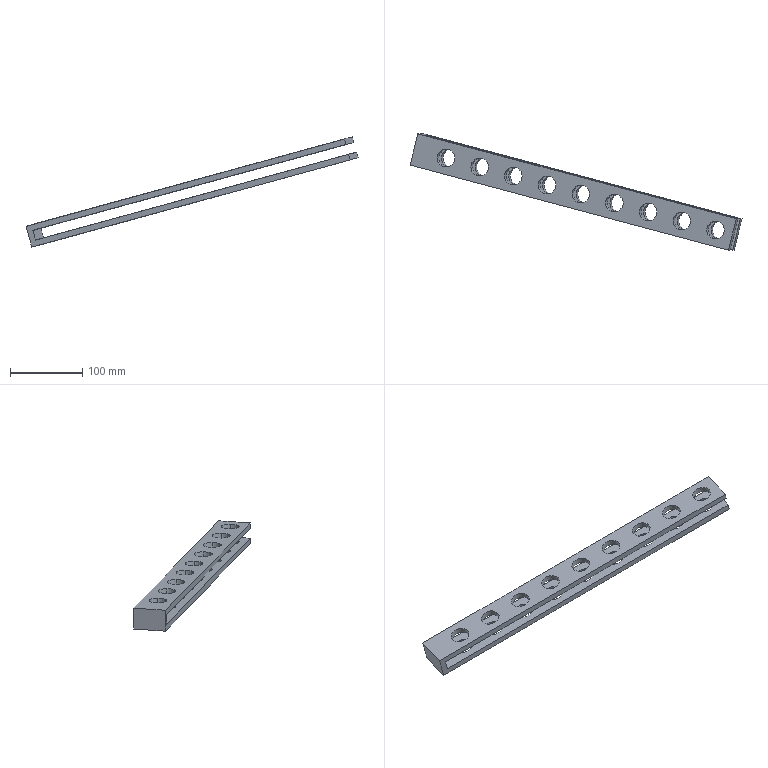Part | SolidWorks | features Cut 2, ExtruThin 1 | 1 solid | 46 faces | box 460.11 x 161.654 x 152.871 mm | volume 274628 mm3 | cylinder 36 | plane 10 | commonest cylinder face diameters 25 x36